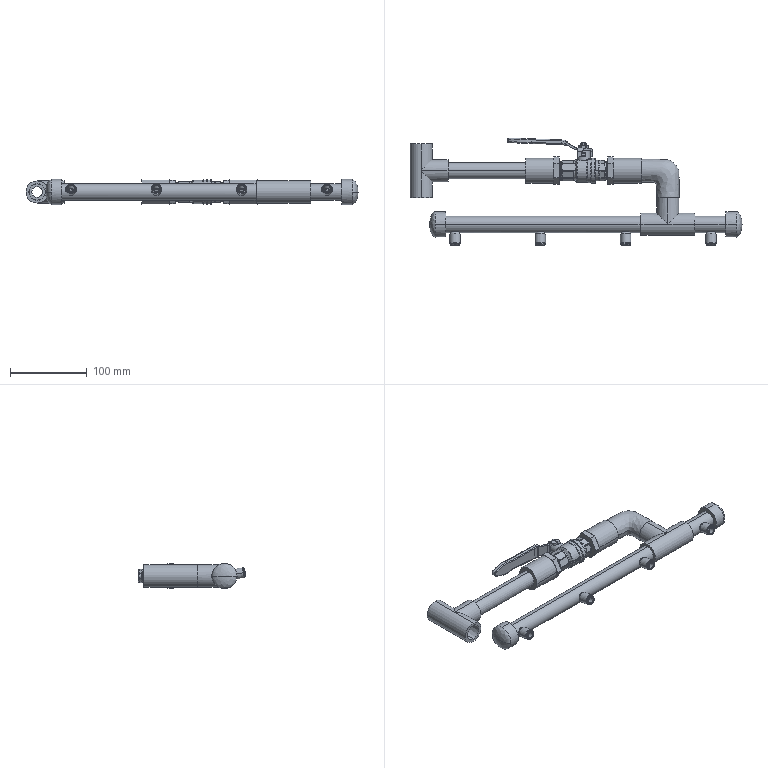Part | SolidWorks | 20 solids | 1144 faces | box 432.043 x 140.383 x 32.766 mm | volume 310066 mm3 | cylinder 286 | spline 279 | plane 267 | cone 209 | sphere 52 | torus 51 | commonest cylinder face diameters 0.635 x62 7 x27 13.868 x24 1.27 x20 2.54 x17 8 x16